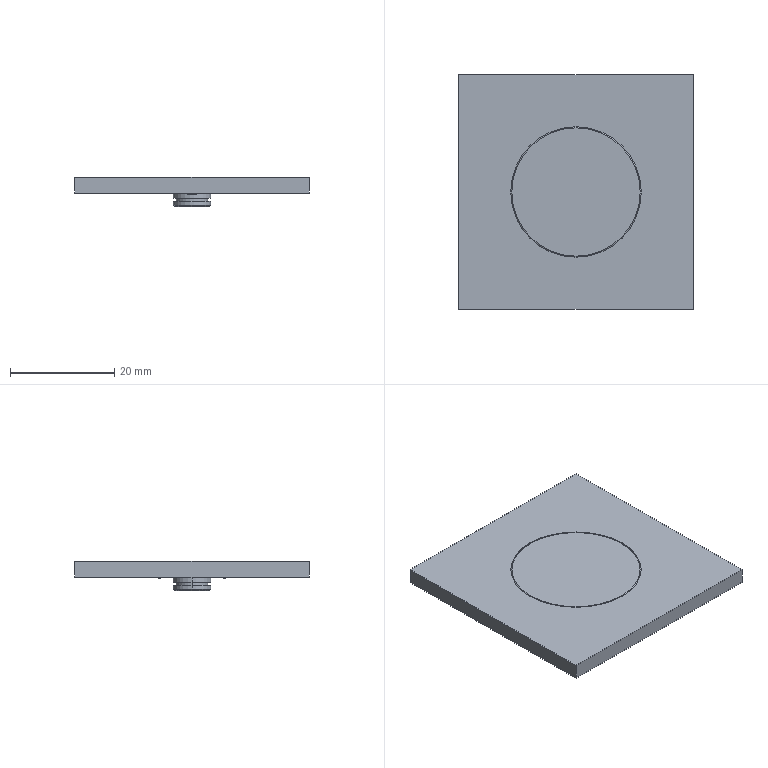NC program | NX | posted with a generic post | part box 45 x 45 x 5.6 mm
Whole program:
N10 G17 G21 G94 G90
(FLOOR_WALL_COPY , TOOL : D10JING)
N12 T14 M6
N14 G54
N16 G17 G0 G90 X-20.5 Y12.497 S9500 M3
N18 G43 Z30. H14
N20 Z6.
N22 G94 G1 Z3. F1250.
N24 X-17.5
N26 X17.5
N28 Y8.298
N30 X-17.5
N32 Y4.098
N34 X17.5
N36 Y-0.101
N38 X-17.5
N40 Y-4.301
N42 X17.5
N44 Y-8.5
N46 X-17.5
N48 X-20.5
N50 Z6.
N52 G0 Z30.
N54 Y12.497
N56 Z5.
N58 G1 Z2.
N60 X-17.5
N62 X17.5
N64 Y8.298
N66 X-17.5
N68 Y4.098
N70 X17.5
N72 Y-0.101
N74 X-17.5
N76 Y-4.301
N78 X17.5
N80 Y-8.5
N82 X-17.5
N84 X-20.5
N86 Z5.
N88 G0 Z30.
N90 Y12.497
N92 Z4.
N94 G1 Z1.
N96 X-17.5
N98 X17.5
N100 Y8.298
N102 X-17.5
N104 Y4.098
N106 X17.5
N108 Y-0.101
N110 X-17.5
N112 Y-4.301
N114 X17.5
N116 Y-8.5
N118 X-17.5
N120 X-20.5
N122 Z4.
N124 G0 Z30.
N126 Y12.497
N128 Z3.
N130 G1 Z0.
N132 X-17.5
N134 X17.5
N136 Y8.298
N138 X-17.5
N140 Y4.098
N142 X17.5
N144 Y-0.101
N146 X-17.5
N148 Y-4.301
N150 X17.5
N152 Y-8.5
N154 X-17.5
N156 X-20.5
N158 Z3.
N160 G0 Z30.
N162 M5
N164 M2